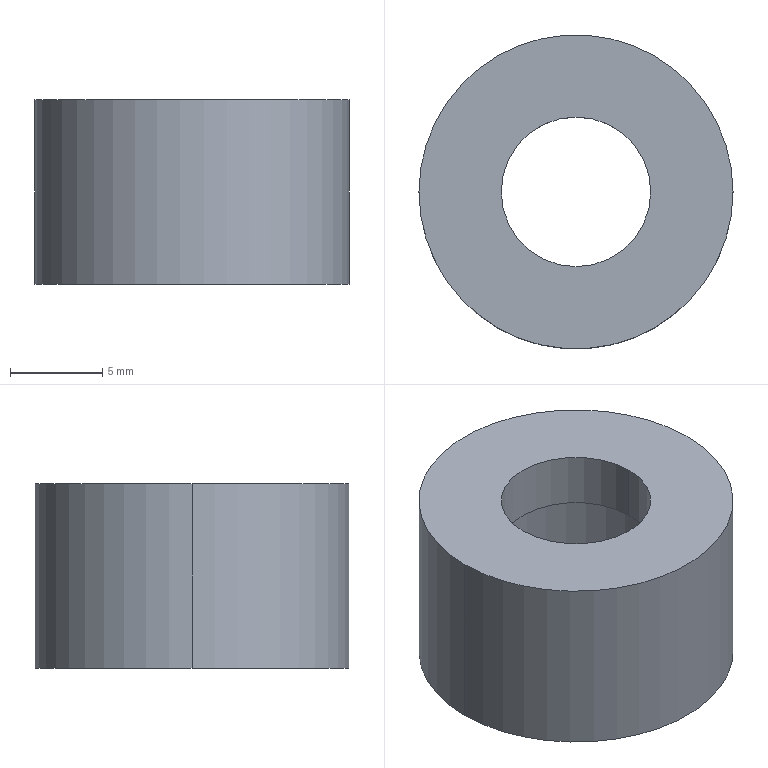Part | SolidWorks | features Cut 1, Extrusion 1 | 1 solid | 9 faces | box 17 x 17 x 10 mm | volume 1256 mm3 | cylinder 6 | plane 3 | commonest cylinder face diameters 8.1 x2 12.5 x2 17 x2
STEP:
#1=CARTESIAN_POINT('',(6.25,0.,7.));
#2=VERTEX_POINT('',#1);
#3=CARTESIAN_POINT('',(-6.25,0.,7.));
#4=VERTEX_POINT('',#3);
#5=CARTESIAN_POINT('',(0.,0.,7.));
#6=DIRECTION('',(0.,0.,-1.));
#7=DIRECTION('',(-1.,0.,0.));
#8=AXIS2_PLACEMENT_3D('',#5,#6,#7);
#9=CIRCLE('',#8,6.25);
#10=EDGE_CURVE('',#2,#4,#9,.T.);
#11=ORIENTED_EDGE('',*,*,#10,.F.);
#12=CARTESIAN_POINT('',(6.25,0.,0.));
#13=VERTEX_POINT('',#12);
#14=CARTESIAN_POINT('',(6.25,0.,7.));
#15=DIRECTION('',(0.,0.,-1.));
#16=VECTOR('',#15,1000.);
#17=LINE('',#14,#16);
#18=EDGE_CURVE('',#2,#13,#17,.T.);
#19=ORIENTED_EDGE('',*,*,#18,.T.);
#20=CARTESIAN_POINT('',(-6.25,0.,0.));
#21=VERTEX_POINT('',#20);
#22=CARTESIAN_POINT('',(0.,0.,0.));
#23=DIRECTION('',(0.,0.,-1.));
#24=DIRECTION('',(-1.,0.,0.));
#25=AXIS2_PLACEMENT_3D('',#22,#23,#24);
#26=CIRCLE('',#25,6.25);
#27=EDGE_CURVE('',#13,#21,#26,.T.);
#28=ORIENTED_EDGE('',*,*,#27,.T.);
#29=CARTESIAN_POINT('',(-6.25,0.,7.));
#30=DIRECTION('',(0.,0.,-1.));
#31=VECTOR('',#30,1000.);
#32=LINE('',#29,#31);
#33=EDGE_CURVE('',#4,#21,#32,.T.);
#34=ORIENTED_EDGE('',*,*,#33,.F.);
#35=EDGE_LOOP('',(#11,#19,#28,#34));
#36=FACE_OUTER_BOUND('',#35,.T.);
#37=CARTESIAN_POINT('',(0.,0.,7.));
#38=DIRECTION('',(0.,0.,-1.));
#39=DIRECTION('',(-1.,0.,0.));
#40=AXIS2_PLACEMENT_3D('',#37,#38,#39);
#41=CYLINDRICAL_SURFACE('',#40,6.25);
#42=ADVANCED_FACE('',(#36),#41,.F.);
#43=CARTESIAN_POINT('',(8.5,0.,10.));
#44=VERTEX_POINT('',#43);
#45=CARTESIAN_POINT('',(-8.5,0.,10.));
#46=VERTEX_POINT('',#45);
#47=CARTESIAN_POINT('',(0.,0.,10.));
#48=DIRECTION('',(0.,0.,1.));
#49=DIRECTION('',(1.,0.,0.));
#50=AXIS2_PLACEMENT_3D('',#47,#48,#49);
#51=CIRCLE('',#50,8.5);
#52=EDGE_CURVE('',#44,#46,#51,.T.);
#53=ORIENTED_EDGE('',*,*,#52,.F.);
#54=CARTESIAN_POINT('',(8.5,0.,0.));
#55=VERTEX_POINT('',#54);
#56=CARTESIAN_POINT('',(8.5,0.,10.));
#57=DIRECTION('',(0.,0.,-1.));
#58=VECTOR('',#57,1000.);
#59=LINE('',#56,#58);
#60=EDGE_CURVE('',#44,#55,#59,.T.);
#61=ORIENTED_EDGE('',*,*,#60,.T.);
#62=CARTESIAN_POINT('',(-8.5,0.,0.));
#63=VERTEX_POINT('',#62);
#64=CARTESIAN_POINT('',(0.,0.,0.));
#65=DIRECTION('',(0.,0.,1.));
#66=DIRECTION('',(1.,0.,0.));
#67=AXIS2_PLACEMENT_3D('',#64,#65,#66);
#68=CIRCLE('',#67,8.5);
#69=EDGE_CURVE('',#55,#63,#68,.T.);
#70=ORIENTED_EDGE('',*,*,#69,.T.);
#71=CARTESIAN_POINT('',(-8.5,0.,10.));
#72=DIRECTION('',(0.,0.,-1.));
#73=VECTOR('',#72,1000.);
#74=LINE('',#71,#73);
#75=EDGE_CURVE('',#46,#63,#74,.T.);
#76=ORIENTED_EDGE('',*,*,#75,.F.);
#77=EDGE_LOOP('',(#53,#61,#70,#76));
#78=FACE_OUTER_BOUND('',#77,.T.);
#79=CARTESIAN_POINT('',(0.,0.,10.));
#80=DIRECTION('',(0.,0.,-1.));
#81=DIRECTION('',(-1.,0.,0.));
#82=AXIS2_PLACEMENT_3D('',#79,#80,#81);
#83=CYLINDRICAL_SURFACE('',#82,8.5);
#84=ADVANCED_FACE('',(#78),#83,.T.);
#85=CARTESIAN_POINT('',(-4.05,0.,10.));
#86=VERTEX_POINT('',#85);
#87=CARTESIAN_POINT('',(4.05,0.,10.));
#88=VERTEX_POINT('',#87);
#89=CARTESIAN_POINT('',(0.,0.,10.));
#90=DIRECTION('',(0.,0.,1.));
#91=DIRECTION('',(1.,0.,0.));
#92=AXIS2_PLACEMENT_3D('',#89,#90,#91);
#93=CIRCLE('',#92,4.05);
#94=EDGE_CURVE('',#86,#88,#93,.T.);
#95=ORIENTED_EDGE('',*,*,#94,.T.);
#96=CARTESIAN_POINT('',(4.05,0.,7.));
#97=VERTEX_POINT('',#96);
#98=CARTESIAN_POINT('',(4.05,0.,10.));
#99=DIRECTION('',(0.,0.,-1.));
#100=VECTOR('',#99,1000.);
#101=LINE('',#98,#100);
#102=EDGE_CURVE('',#88,#97,#101,.T.);
#103=ORIENTED_EDGE('',*,*,#102,.T.);
#104=CARTESIAN_POINT('',(-4.05,0.,7.));
#105=VERTEX_POINT('',#104);
#106=CARTESIAN_POINT('',(0.,0.,7.));
#107=DIRECTION('',(0.,0.,-1.));
#108=DIRECTION('',(-1.,0.,0.));
#109=AXIS2_PLACEMENT_3D('',#106,#107,#108);
#110=CIRCLE('',#109,4.05);
#111=EDGE_CURVE('',#97,#105,#110,.T.);
#112=ORIENTED_EDGE('',*,*,#111,.T.);
#113=CARTESIAN_POINT('',(-4.05,0.,10.));
#114=DIRECTION('',(0.,0.,-1.));
#115=VECTOR('',#114,1000.);
#116=LINE('',#113,#115);
#117=EDGE_CURVE('',#86,#105,#116,.T.);
#118=ORIENTED_EDGE('',*,*,#117,.F.);
#119=EDGE_LOOP('',(#95,#103,#112,#118));
#120=FACE_OUTER_BOUND('',#119,.T.);
#121=CARTESIAN_POINT('',(0.,0.,10.));
#122=DIRECTION('',(0.,0.,-1.));
#123=DIRECTION('',(-1.,0.,0.));
#124=AXIS2_PLACEMENT_3D('',#121,#122,#123);
#125=CYLINDRICAL_SURFACE('',#124,4.05);
#126=ADVANCED_FACE('',(#120),#125,.F.);
#127=ORIENTED_EDGE('',*,*,#102,.F.);
#128=CARTESIAN_POINT('',(0.,0.,10.));
#129=DIRECTION('',(0.,0.,1.));
#130=DIRECTION('',(1.,0.,0.));
#131=AXIS2_PLACEMENT_3D('',#128,#129,#130);
#132=CIRCLE('',#131,4.05);
#133=EDGE_CURVE('',#88,#86,#132,.T.);
#134=ORIENTED_EDGE('',*,*,#133,.T.);
#135=ORIENTED_EDGE('',*,*,#117,.T.);
#136=CARTESIAN_POINT('',(0.,0.,7.));
#137=DIRECTION('',(0.,0.,-1.));
#138=DIRECTION('',(-1.,0.,0.));
#139=AXIS2_PLACEMENT_3D('',#136,#137,#138);
#140=CIRCLE('',#139,4.05);
#141=EDGE_CURVE('',#105,#97,#140,.T.);
#142=ORIENTED_EDGE('',*,*,#141,.T.);
#143=EDGE_LOOP('',(#127,#134,#135,#142));
#144=FACE_OUTER_BOUND('',#143,.T.);
#145=CARTESIAN_POINT('',(0.,0.,10.));
#146=DIRECTION('',(0.,0.,-1.));
#147=DIRECTION('',(-1.,0.,0.));
#148=AXIS2_PLACEMENT_3D('',#145,#146,#147);
#149=CYLINDRICAL_SURFACE('',#148,4.05);
#150=ADVANCED_FACE('',(#144),#149,.F.);
#151=CARTESIAN_POINT('',(0.,0.,10.));
#152=DIRECTION('',(0.,0.,1.));
#153=DIRECTION('',(1.,0.,0.));
#154=AXIS2_PLACEMENT_3D('',#151,#152,#153);
#155=CIRCLE('',#154,8.5);
#156=EDGE_CURVE('',#46,#44,#155,.T.);
#157=ORIENTED_EDGE('',*,*,#156,.T.);
#158=ORIENTED_EDGE('',*,*,#52,.T.);
#159=EDGE_LOOP('',(#157,#158));
#160=FACE_OUTER_BOUND('',#159,.T.);
#161=ORIENTED_EDGE('',*,*,#94,.F.);
#162=ORIENTED_EDGE('',*,*,#133,.F.);
#163=EDGE_LOOP('',(#161,#162));
#164=FACE_BOUND('',#163,.T.);
#165=CARTESIAN_POINT('',(0.,0.,10.));
#166=DIRECTION('',(0.,0.,1.));
#167=DIRECTION('',(1.,0.,0.));
#168=AXIS2_PLACEMENT_3D('',#165,#166,#167);
#169=PLANE('',#168);
#170=ADVANCED_FACE('',(#160,#164),#169,.T.);
#171=CARTESIAN_POINT('',(0.,0.,0.));
#172=DIRECTION('',(0.,0.,-1.));
#173=DIRECTION('',(-1.,0.,0.));
#174=AXIS2_PLACEMENT_3D('',#171,#172,#173);
#175=CIRCLE('',#174,6.25);
#176=EDGE_CURVE('',#21,#13,#175,.T.);
#177=ORIENTED_EDGE('',*,*,#176,.F.);
#178=ORIENTED_EDGE('',*,*,#27,.F.);
#179=EDGE_LOOP('',(#177,#178));
#180=FACE_BOUND('',#179,.T.);
#181=CARTESIAN_POINT('',(0.,0.,0.));
#182=DIRECTION('',(0.,0.,1.));
#183=DIRECTION('',(1.,0.,0.));
#184=AXIS2_PLACEMENT_3D('',#181,#182,#183);
#185=CIRCLE('',#184,8.5);
#186=EDGE_CURVE('',#63,#55,#185,.T.);
#187=ORIENTED_EDGE('',*,*,#186,.F.);
#188=ORIENTED_EDGE('',*,*,#69,.F.);
#189=EDGE_LOOP('',(#187,#188));
#190=FACE_OUTER_BOUND('',#189,.T.);
#191=CARTESIAN_POINT('',(0.,0.,0.));
#192=DIRECTION('',(0.,0.,1.));
#193=DIRECTION('',(1.,0.,0.));
#194=AXIS2_PLACEMENT_3D('',#191,#192,#193);
#195=PLANE('',#194);
#196=ADVANCED_FACE('',(#180,#190),#195,.F.);
#197=ORIENTED_EDGE('',*,*,#60,.F.);
#198=ORIENTED_EDGE('',*,*,#156,.F.);
#199=ORIENTED_EDGE('',*,*,#75,.T.);
#200=ORIENTED_EDGE('',*,*,#186,.T.);
#201=EDGE_LOOP('',(#197,#198,#199,#200));
#202=FACE_OUTER_BOUND('',#201,.T.);
#203=CARTESIAN_POINT('',(0.,0.,10.));
#204=DIRECTION('',(0.,0.,-1.));
#205=DIRECTION('',(-1.,0.,0.));
#206=AXIS2_PLACEMENT_3D('',#203,#204,#205);
#207=CYLINDRICAL_SURFACE('',#206,8.5);
#208=ADVANCED_FACE('',(#202),#207,.T.);
#209=ORIENTED_EDGE('',*,*,#18,.F.);
#210=CARTESIAN_POINT('',(0.,0.,7.));
#211=DIRECTION('',(0.,0.,-1.));
#212=DIRECTION('',(-1.,0.,0.));
#213=AXIS2_PLACEMENT_3D('',#210,#211,#212);
#214=CIRCLE('',#213,6.25);
#215=EDGE_CURVE('',#4,#2,#214,.T.);
#216=ORIENTED_EDGE('',*,*,#215,.F.);
#217=ORIENTED_EDGE('',*,*,#33,.T.);
#218=ORIENTED_EDGE('',*,*,#176,.T.);
#219=EDGE_LOOP('',(#209,#216,#217,#218));
#220=FACE_OUTER_BOUND('',#219,.T.);
#221=CARTESIAN_POINT('',(0.,0.,7.));
#222=DIRECTION('',(0.,0.,-1.));
#223=DIRECTION('',(-1.,0.,0.));
#224=AXIS2_PLACEMENT_3D('',#221,#222,#223);
#225=CYLINDRICAL_SURFACE('',#224,6.25);
#226=ADVANCED_FACE('',(#220),#225,.F.);
#227=ORIENTED_EDGE('',*,*,#141,.F.);
#228=ORIENTED_EDGE('',*,*,#111,.F.);
#229=EDGE_LOOP('',(#227,#228));
#230=FACE_BOUND('',#229,.T.);
#231=ORIENTED_EDGE('',*,*,#215,.T.);
#232=ORIENTED_EDGE('',*,*,#10,.T.);
#233=EDGE_LOOP('',(#231,#232));
#234=FACE_OUTER_BOUND('',#233,.T.);
#235=CARTESIAN_POINT('',(0.,0.,7.));
#236=DIRECTION('',(0.,0.,-1.));
#237=DIRECTION('',(-1.,0.,0.));
#238=AXIS2_PLACEMENT_3D('',#235,#236,#237);
#239=PLANE('',#238);
#240=ADVANCED_FACE('',(#230,#234),#239,.T.);
#241=CLOSED_SHELL('',(#42,#84,#126,#150,#170,#196,#208,#226,#240));
#242=MANIFOLD_SOLID_BREP('',#241);
#243=CARTESIAN_POINT('',(0.,0.,0.));
#244=DIRECTION('',(0.,0.,1.));
#245=DIRECTION('',(1.,0.,0.));
#246=AXIS2_PLACEMENT_3D('',#243,#244,#245);
#247=(LENGTH_UNIT()NAMED_UNIT(*)SI_UNIT(.MILLI.,.METRE.));
#248=UNCERTAINTY_MEASURE_WITH_UNIT(LENGTH_MEASURE(0.00001),#247,'','');
#249=(NAMED_UNIT(*)PLANE_ANGLE_UNIT()SI_UNIT($,.RADIAN.));
#250=(NAMED_UNIT(*)SI_UNIT($,.STERADIAN.)SOLID_ANGLE_UNIT());
#251=(GEOMETRIC_REPRESENTATION_CONTEXT(3)GLOBAL_UNCERTAINTY_ASSIGNED_CONTEXT((#248))GLOBAL_UNIT_ASSIGNED_CONTEXT((#247,#249,#250))REPRESENTATION_CONTEXT('',''));
#252=ADVANCED_BREP_SHAPE_REPRESENTATION('',(#242,#246),#251);